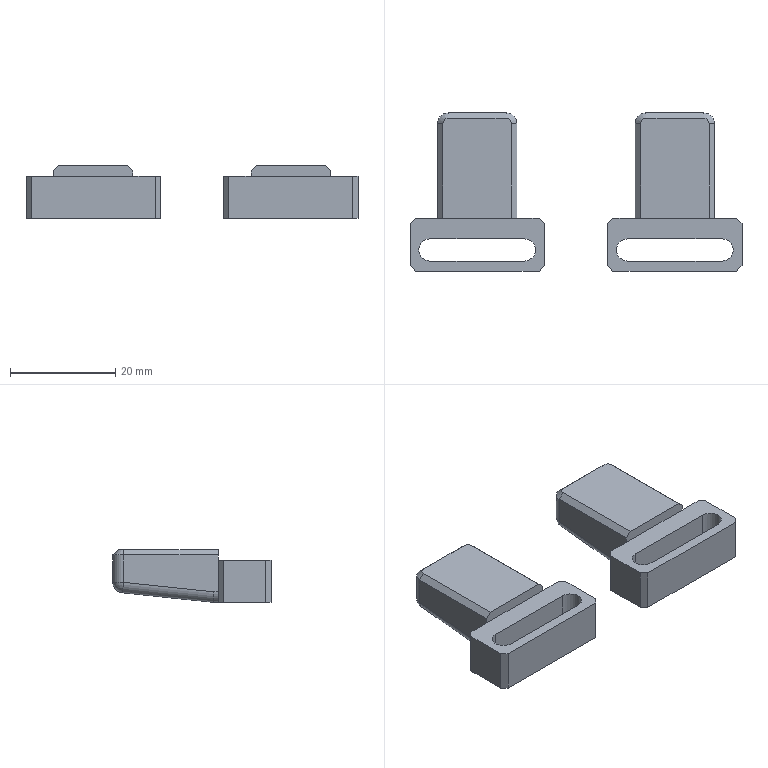NC program | NX | posted with a generic post | part box 63 x 30 x 10 mm
Lines 14606 to 15440 of 24780:
(FIXED_CONTOUR_COPY , TOOL : R2)
N29192 T18 M6
N29194 G54
N29196 G17 G0 G90 X21.594 Y2.999 B0. C0. S9500 M3
N29198 G43 Z30. H18
N29200 Z2.8
N29202 G94 G1 Z-1.939 F1000.
N29204 X21.607 Y2.986 Z-1.906 F2500.
N29206 X21.67 Y2.923 Z-1.669
N29208 X21.669 Y2.857 Z-1.674
N29210 X21.607 Y2.919 Z-1.906
N29212 X21.525 Y3. Z-2.113
N29214 X21.495 Z-2.188
N29216 X21.462 Z-2.252
N29218 Z-2.267
N29220 X21.547 Y2.915 Z-2.061
N29222 X21.607 Y2.855 Z-1.907
N29224 X21.668 Y2.794 Z-1.678
N29226 X21.667 Y2.75 Z-1.68
N29228 X21.607 Y2.811 Z-1.907
N29230 X21.553 Y2.864 Z-2.046
N29232 X21.443 Y2.974 Z-2.311
N29234 X21.418 Y3. Z-2.357
N29236 Z-2.339
N29238 X21.329 Z-2.512
N29240 Y2.999 Z-2.515
N29242 X21.443 Y2.884 Z-2.311
N29244 X21.49 Y2.837 Z-2.199
N29246 X21.565 Y2.762 Z-2.016
N29248 X21.604 Y2.724 Z-1.915
N29250 X21.666 Y2.662 Z-1.686
N29252 X21.665 Y2.596 Z-1.69
N29254 X21.622 Y2.639 Z-1.85
N29256 X21.597 Y2.664 Z-1.932
N29258 X21.566 Y2.695 Z-2.013
N29260 X21.466 Y2.795 Z-2.259
N29262 X21.443 Y2.818 Z-2.311
N29264 X21.284 Y2.977 Z-2.594
N29266 X21.261 Y3. Z-2.627
N29268 Z-2.618
N29270 X21.204 Z-2.701
N29272 Z-2.709
N29274 X21.281 Y2.923 Z-2.599
N29276 X21.443 Y2.761 Z-2.311
N29278 X21.466 Y2.738 Z-2.259
N29280 X21.566 Y2.638 Z-2.014
N29282 X21.592 Y2.613 Z-1.947
N29284 X21.631 Y2.573 Z-1.817
N29286 X21.664 Y2.54 Z-1.694
N29288 X21.663 Y2.438 Z-1.7
N29290 X21.648 Y2.453 Z-1.756
N29292 X21.582 Y2.52 Z-1.973
N29294 X21.466 Y2.635 Z-2.26
N29296 X21.449 Y2.652 Z-2.299
N29298 X21.276 Y2.825 Z-2.609
N29300 X21.194 Y2.907 Z-2.724
N29302 X21.101 Y3. Z-2.85
N29304 Z-2.846
N29306 X21.038 Z-2.92
N29308 Z-2.927
N29310 X21.078 Y2.96 Z-2.881
N29312 X21.194 Y2.844 Z-2.724
N29314 X21.273 Y2.765 Z-2.614
N29316 X21.396 Y2.642 Z-2.393
N29318 X21.453 Y2.585 Z-2.29
N29320 X21.575 Y2.463 Z-1.989
N29322 X21.662 Y2.376 Z-1.704
N29324 X21.66 Y2.273 Z-1.71
N29326 X21.564 Y2.37 Z-2.019
N29328 X21.459 Y2.474 Z-2.276
N29330 X21.369 Y2.564 Z-2.443
N29332 X21.272 Y2.661 Z-2.615
N29334 X21.191 Y2.742 Z-2.728
N29336 X21.078 Y2.855 Z-2.881
N29338 X20.988 Y2.945 Z-2.986
N29340 X20.935 Y2.998 Z-3.042
N29342 X20.898 Z-3.08
N29344 X20.839 Y3. Z-3.136
N29346 Z-3.142
N29348 X20.988 Y2.851 Z-2.986
N29350 X21.078 Y2.761 Z-2.881
N29352 X21.272 Y2.567 Z-2.615
N29354 X21.369 Y2.47 Z-2.443
N29356 X21.465 Y2.374 Z-2.264
N29358 X21.563 Y2.276 Z-2.021
N29360 X21.659 Y2.18 Z-1.716
N29362 X21.657 Y2.078 Z-1.723
N29364 X21.562 Y2.173 Z-2.023
N29366 X21.466 Y2.269 Z-2.262
N29368 X21.369 Y2.366 Z-2.443
N29370 X21.272 Y2.463 Z-2.615
N29372 X21.078 Y2.657 Z-2.881
N29374 X20.987 Y2.748 Z-2.987
N29376 X20.788 Y2.947 Z-3.196
N29378 X20.735 Y3. Z-3.239
N29380 X20.633 Y2.998 Z-3.323
N29382 X20.788 Y2.843 Z-3.196
N29384 X20.966 Y2.666 Z-3.01
N29386 X21.078 Y2.553 Z-2.881
N29388 X21.272 Y2.359 Z-2.615
N29390 X21.399 Y2.232 Z-2.388
N29392 X21.466 Y2.165 Z-2.262
N29394 X21.562 Y2.07 Z-2.025
N29396 X21.656 Y1.975 Z-1.729
N29398 X21.654 Y1.872 Z-1.736
N29400 X21.561 Y1.966 Z-2.026
N29402 X21.466 Y2.06 Z-2.263
N29404 X21.369 Y2.157 Z-2.443
N29406 X21.272 Y2.254 Z-2.615
N29408 X21.078 Y2.449 Z-2.881
N29410 X20.944 Y2.583 Z-3.032
N29412 X20.786 Y2.741 Z-3.198
N29414 X20.548 Y2.978 Z-3.392
N29416 X20.528 Y2.998 Z-3.407
N29418 X20.507 Y3. Z-3.422
N29420 X20.434 Z-3.468
N29422 Z-3.474
N29424 X20.548 Y2.885 Z-3.392
N29426 X20.767 Y2.666 Z-3.213
N29428 X20.822 Y2.611 Z-3.16
N29430 X20.925 Y2.509 Z-3.053
N29432 X21.078 Y2.355 Z-2.88
N29434 X21.272 Y2.161 Z-2.616
N29436 X21.369 Y2.064 Z-2.443
N29438 X21.466 Y1.967 Z-2.264
N29440 X21.56 Y1.873 Z-2.028
N29442 X21.653 Y1.781 Z-1.742
N29444 X21.652 Y1.697 Z-1.747
N29446 X21.56 Y1.789 Z-2.03
N29448 X21.466 Y1.883 Z-2.264
N29450 X21.369 Y1.98 Z-2.443
N29452 X21.272 Y2.077 Z-2.616
N29454 X21.078 Y2.271 Z-2.881
N29456 X20.907 Y2.442 Z-3.071
N29458 X20.849 Y2.5 Z-3.132
N29460 X20.75 Y2.598 Z-3.227
N29462 X20.548 Y2.8 Z-3.392
N29464 X20.471 Y2.878 Z-3.45
N29466 X20.349 Y3. Z-3.527
N29468 Z-3.52
N29470 X20.264 Z-3.573
N29472 Z-3.58
N29474 X20.492 Y2.772 Z-3.437
N29476 X20.734 Y2.53 Z-3.241
N29478 X20.889 Y2.375 Z-3.09
N29480 X21.078 Y2.186 Z-2.881
N29482 X21.272 Y1.992 Z-2.616
N29484 X21.389 Y1.875 Z-2.406
N29486 X21.466 Y1.798 Z-2.264
N29488 X21.559 Y1.705 Z-2.031
N29490 X21.65 Y1.614 Z-1.752
N29492 X21.649 Y1.511 Z-1.759
N29494 X21.558 Y1.601 Z-2.033
N29496 X21.466 Y1.694 Z-2.265
N29498 X21.369 Y1.791 Z-2.443
N29500 X21.272 Y1.888 Z-2.616
N29502 X21.078 Y2.082 Z-2.881
N29504 X20.884 Y2.276 Z-3.095
N29506 X20.713 Y2.447 Z-3.258
N29508 X20.496 Y2.664 Z-3.435
N29510 X20.189 Y2.971 Z-3.627
N29512 X20.16 Y3. Z-3.641
N29514 Z-3.638
N29516 X20.131 Y2.998 Z-3.654
N29518 X20.056 Y3. Z-3.688
N29520 Z-3.69
N29522 X20.189 Y2.867 Z-3.627
N29524 X20.496 Y2.56 Z-3.435
N29526 X20.701 Y2.354 Z-3.266
N29528 X20.884 Y2.171 Z-3.095
N29530 X21.078 Y1.977 Z-2.881
N29532 X21.272 Y1.783 Z-2.616
N29534 X21.369 Y1.686 Z-2.443
N29536 X21.466 Y1.589 Z-2.265
N29538 X21.558 Y1.498 Z-2.035
N29540 X21.647 Y1.408 Z-1.765
N29542 X21.646 Y1.319 Z-1.771
N29544 X21.557 Y1.408 Z-2.036
N29546 X21.466 Y1.499 Z-2.265
N29548 X21.369 Y1.596 Z-2.443
N29550 X21.272 Y1.693 Z-2.616
N29552 X21.078 Y1.887 Z-2.881
N29554 X20.884 Y2.081 Z-3.095
N29556 X20.69 Y2.275 Z-3.276
N29558 X20.496 Y2.469 Z-3.435
N29560 X20.189 Y2.776 Z-3.627
N29562 X19.965 Y3. Z-3.732
N29564 Z-3.726
N29566 X19.874 Z-3.765
N29568 Z-3.774
N29570 X20.178 Y2.696 Z-3.633
N29572 X20.215 Y2.659 Z-3.611
N29574 X20.496 Y2.378 Z-3.435
N29576 X20.69 Y2.184 Z-3.276
N29578 X20.884 Y1.99 Z-3.095
N29580 X21.078 Y1.796 Z-2.881
N29582 X21.272 Y1.602 Z-2.616
N29584 X21.369 Y1.505 Z-2.443
N29586 X21.466 Y1.408 Z-2.266
N29588 X21.556 Y1.318 Z-2.038
N29590 X21.645 Y1.229 Z-1.776
N29592 X21.643 Y1.127 Z-1.783
N29594 X21.555 Y1.215 Z-2.04
N29596 X21.466 Y1.304 Z-2.266
N29598 X21.338 Y1.432 Z-2.499
N29600 X21.272 Y1.498 Z-2.616
N29602 X21.078 Y1.692 Z-2.881
N29604 X20.884 Y1.886 Z-3.095
N29606 X20.69 Y2.08 Z-3.276
N29608 X20.496 Y2.274 Z-3.435
N29610 X20.257 Y2.513 Z-3.585
N29612 X20.16 Y2.61 Z-3.641
N29614 X19.914 Y2.856 Z-3.757
N29616 X19.824 Y2.946 Z-3.796
N29618 X19.77 Y3. Z-3.813
N29620 Z-3.809
N29622 X19.737 Y2.998 Z-3.824
N29624 X19.711 Y3. Z-3.832
N29626 X19.667 Z-3.843
N29628 Z-3.846
N29630 X19.824 Y2.842 Z-3.796
N29632 X19.915 Y2.751 Z-3.756
N29634 X20.142 Y2.524 Z-3.65
N29636 X20.298 Y2.368 Z-3.559
N29638 X20.496 Y2.17 Z-3.435
N29640 X20.69 Y1.976 Z-3.276
N29642 X20.884 Y1.782 Z-3.095
N29644 X21.078 Y1.588 Z-2.881
N29646 X21.272 Y1.394 Z-2.616
N29648 X21.466 Y1.2 Z-2.266
N29650 X21.555 Y1.112 Z-2.042
N29652 X21.642 Y1.024 Z-1.789
N29654 X21.64 Y0.931 Z-1.795
N29656 X21.554 Y1.017 Z-2.044
N29658 X21.466 Y1.105 Z-2.266
N29660 X21.272 Y1.299 Z-2.617
N29662 X21.078 Y1.493 Z-2.881
N29664 X20.884 Y1.687 Z-3.095
N29666 X20.69 Y1.881 Z-3.276
N29668 X20.496 Y2.075 Z-3.435
N29670 X20.302 Y2.269 Z-3.556
N29672 X20.126 Y2.445 Z-3.657
N29674 X19.914 Y2.657 Z-3.757
N29676 X19.883 Y2.688 Z-3.768
N29678 X19.823 Y2.748 Z-3.796
N29680 X19.571 Y3. Z-3.877
N29682 Z-3.869
N29684 X19.475 Z-3.895
N29686 Z-3.904
N29688 X19.526 Y2.949 Z-3.892
N29690 X19.803 Y2.672 Z-3.803
N29692 X19.851 Y2.623 Z-3.78
N29694 X19.914 Y2.561 Z-3.757
N29696 X20.12 Y2.354 Z-3.659
N29698 X20.302 Y2.173 Z-3.556
N29700 X20.496 Y1.979 Z-3.435
N29702 X20.69 Y1.785 Z-3.276
N29704 X20.884 Y1.591 Z-3.095
N29706 X21.078 Y1.397 Z-2.881
N29708 X21.272 Y1.203 Z-2.617
N29710 X21.466 Y1.008 Z-2.266
N29712 X21.553 Y0.922 Z-2.045
N29714 X21.639 Y0.836 Z-1.801
N29716 X21.638 Y0.733 Z-1.808
N29718 X21.552 Y0.819 Z-2.047
N29720 X21.466 Y0.905 Z-2.266
N29722 X21.272 Y1.099 Z-2.617
N29724 X21.078 Y1.293 Z-2.881
N29726 X20.884 Y1.487 Z-3.095
N29728 X20.69 Y1.681 Z-3.276
N29730 X20.496 Y1.875 Z-3.435
N29732 X20.302 Y2.069 Z-3.556
N29734 X20.108 Y2.263 Z-3.666
N29736 X19.914 Y2.457 Z-3.757
N29738 X19.817 Y2.554 Z-3.793
N29740 X19.781 Y2.59 Z-3.809
N29742 X19.526 Y2.845 Z-3.892
N29744 X19.436 Y2.935 Z-3.914
N29746 X19.371 Y3. Z-3.926
N29748 Z-3.923
N29750 X19.342 Y2.998 Z-3.931
N29752 X19.307 Y3. Z-3.938
N29754 X19.268 Z-3.943
N29756 Z-3.945
N29758 X19.436 Y2.832 Z-3.914
N29760 X19.526 Y2.742 Z-3.892
N29762 X19.76 Y2.508 Z-3.816
N29764 X19.783 Y2.484 Z-3.806
N29766 X19.914 Y2.353 Z-3.756
N29768 X20.108 Y2.16 Z-3.666
N29770 X20.302 Y1.966 Z-3.556
N29772 X20.496 Y1.772 Z-3.435
N29774 X20.69 Y1.578 Z-3.276
N29776 X20.884 Y1.383 Z-3.095
N29778 X21.078 Y1.189 Z-2.881
N29780 X21.272 Y0.995 Z-2.617
N29782 X21.466 Y0.801 Z-2.266
N29784 X21.552 Y0.716 Z-2.049
N29786 X21.636 Y0.631 Z-1.814
N29788 X21.635 Y0.535 Z-1.82
N29790 X21.551 Y0.618 Z-2.051
N29792 X21.466 Y0.703 Z-2.266
N29794 X21.272 Y0.897 Z-2.618
N29796 X21.078 Y1.091 Z-2.881
N29798 X20.884 Y1.285 Z-3.095
N29800 X20.69 Y1.479 Z-3.276
N29802 X20.496 Y1.673 Z-3.435
N29804 X20.302 Y1.867 Z-3.556
N29806 X20.108 Y2.061 Z-3.666
N29808 X19.914 Y2.256 Z-3.757
N29810 X19.739 Y2.43 Z-3.823
N29812 X19.526 Y2.644 Z-3.892
N29814 X19.432 Y2.737 Z-3.914
N29816 X19.17 Y3. Z-3.964
N29818 Z-3.958
N29820 X19.071 Z-3.973
N29822 Z-3.978
N29824 X19.138 Y2.933 Z-3.97
N29826 X19.411 Y2.659 Z-3.918
N29828 X19.526 Y2.545 Z-3.892
N29830 X19.72 Y2.351 Z-3.829
N29832 X19.914 Y2.157 Z-3.757
N29834 X20.108 Y1.963 Z-3.666
N29836 X20.302 Y1.768 Z-3.556
N29838 X20.496 Y1.574 Z-3.435
N29840 X20.69 Y1.38 Z-3.276
N29842 X20.884 Y1.186 Z-3.095
N29844 X21.078 Y0.992 Z-2.881
N29846 X21.272 Y0.798 Z-2.618
N29848 X21.466 Y0.604 Z-2.266
N29850 X21.55 Y0.52 Z-2.053
N29852 X21.633 Y0.437 Z-1.827
N29854 X21.632 Y0.335 Z-1.833
N29856 X21.549 Y0.417 Z-2.055
N29858 X21.466 Y0.501 Z-2.266
N29860 X21.272 Y0.695 Z-2.618
N29862 X21.078 Y0.889 Z-2.881
N29864 X20.884 Y1.083 Z-3.095
N29866 X20.69 Y1.277 Z-3.276
N29868 X20.496 Y1.471 Z-3.435
N29870 X20.302 Y1.665 Z-3.556
N29872 X20.108 Y1.859 Z-3.666
N29874 X19.914 Y2.053 Z-3.757
N29876 X19.72 Y2.247 Z-3.829
N29878 X19.526 Y2.441 Z-3.892
N29880 X19.39 Y2.577 Z-3.922
N29882 X19.138 Y2.829 Z-3.97
N29884 X18.967 Y3. Z-3.99
N29886 X18.918 Z-3.992
N29888 X18.863
N29890 Z-3.995
N29892 X18.985 Y2.877 Z-3.989
N29894 X19.138 Y2.725 Z-3.97
N29896 X19.368 Y2.494 Z-3.926
N29898 X19.526 Y2.337 Z-3.892
N29900 X19.72 Y2.143 Z-3.829
N29902 X19.914 Y1.949 Z-3.757
N29904 X20.108 Y1.755 Z-3.666
N29906 X20.303 Y1.56 Z-3.556
N29908 X20.496 Y1.367 Z-3.435
N29910 X20.69 Y1.173 Z-3.276
N29912 X20.884 Y0.979 Z-3.095
N29914 X21.078 Y0.785 Z-2.881
N29916 X21.272 Y0.591 Z-2.618
N29918 X21.466 Y0.397 Z-2.266
N29920 X21.549 Y0.314 Z-2.058
N29922 X21.63 Y0.233 Z-1.839
N29924 X21.628 Y0.135 Z-1.845
N29926 X21.548 Y0.215 Z-2.061
N29928 X21.466 Y0.297 Z-2.266
N29930 X21.272 Y0.491 Z-2.618
N29932 X21.078 Y0.685 Z-2.881
N29934 X20.884 Y0.879 Z-3.095
N29936 X20.69 Y1.073 Z-3.276
N29938 X20.496 Y1.267 Z-3.435
N29940 X20.302 Y1.461 Z-3.556
N29942 X20.108 Y1.655 Z-3.666
N29944 X19.914 Y1.849 Z-3.757
N29946 X19.72 Y2.043 Z-3.829
N29948 X19.526 Y2.237 Z-3.892
N29950 X19.348 Y2.415 Z-3.93
N29952 X19.138 Y2.625 Z-3.97
N29954 X18.953 Y2.81 Z-3.992
N29956 X18.763 Y3. Z-3.999
N29958 Z-3.992
N29960 X18.663
N29962 Z-3.996
N29964 X18.749 Y2.913 Z-3.999
N29966 X18.943 Y2.719 Z-3.993
N29968 X19.138 Y2.525 Z-3.97
N29970 X19.332 Y2.331 Z-3.933
N29972 X19.526 Y2.137 Z-3.892
N29974 X19.72 Y1.943 Z-3.829
N29976 X19.914 Y1.749 Z-3.757
N29978 X20.108 Y1.555 Z-3.666
N29980 X20.302 Y1.361 Z-3.556
N29982 X20.496 Y1.167 Z-3.435
N29984 X20.69 Y0.973 Z-3.276
N29986 X20.884 Y0.779 Z-3.095
N29988 X21.078 Y0.585 Z-2.881
N29990 X21.272 Y0.391 Z-2.619
N29992 X21.466 Y0.197 Z-2.266
N29994 X21.547 Y0.116 Z-2.064
N29996 X21.626 Y0.037 Z-1.852
N29998 X21.624 Y-0.066 Z-1.858
N30000 X21.535 Y0.023 Z-2.094
N30002 X21.466 Y0.091 Z-2.266
N30004 X21.272 Y0.286 Z-2.619
N30006 X21.078 Y0.48 Z-2.881
N30008 X20.884 Y0.674 Z-3.095
N30010 X20.69 Y0.868 Z-3.276
N30012 X20.496 Y1.062 Z-3.435
N30014 X20.302 Y1.256 Z-3.556
N30016 X20.108 Y1.45 Z-3.666
N30018 X19.914 Y1.644 Z-3.757
N30020 X19.72 Y1.838 Z-3.829
N30022 X19.526 Y2.032 Z-3.892
N30024 X19.332 Y2.226 Z-3.933
N30026 X19.138 Y2.42 Z-3.97
N30028 X18.943 Y2.614 Z-3.993
N30030 X18.749 Y2.808 Z-3.999
N30032 X18.559 Y2.998 Z-3.991
N30034 X18.532 Y3. Z-3.989
N30036 X18.452 Z-3.977
N30038 Z-3.981
N30040 X18.526 Y2.926 Z-3.99
N30042 X18.656 Y2.796 Z-3.996
N30044 X18.749 Y2.703 Z-3.999
N30046 X18.958 Y2.494 Z-3.991
N30048 X19.138 Y2.315 Z-3.97
N30050 X19.332 Y2.121 Z-3.933
N30052 X19.526 Y1.926 Z-3.892
N30054 X19.72 Y1.732 Z-3.829
N30056 X19.914 Y1.538 Z-3.757
N30058 X20.108 Y1.344 Z-3.666
N30060 X20.302 Y1.15 Z-3.556
N30062 X20.496 Y0.956 Z-3.435
N30064 X20.69 Y0.762 Z-3.276
N30066 X20.884 Y0.568 Z-3.095
N30068 X21.078 Y0.374 Z-2.881
N30070 X21.272 Y0.18 Z-2.619
N30072 X21.466 Y-0.014 Z-2.266
N30074 X21.559 Y-0.107 Z-2.032
N30076 X21.622 Y-0.169 Z-1.865
N30078 X21.62 Y-0.273 Z-1.871
N30080 X21.544 Y-0.197 Z-2.074
N30082 X21.466 Y-0.12 Z-2.266
N30084 X21.272 Y0.074 Z-2.619
N30086 X21.078 Y0.268 Z-2.881
N30088 X20.884 Y0.463 Z-3.095
N30090 X20.69 Y0.657 Z-3.276
N30092 X20.496 Y0.851 Z-3.435
N30094 X20.302 Y1.045 Z-3.556
N30096 X20.108 Y1.239 Z-3.666
N30098 X19.914 Y1.433 Z-3.757
N30100 X19.72 Y1.627 Z-3.829
N30102 X19.526 Y1.821 Z-3.892
N30104 X19.332 Y2.015 Z-3.933
N30106 X19.138 Y2.209 Z-3.97
N30108 X18.943 Y2.403 Z-3.993
N30110 X18.749 Y2.597 Z-3.999
N30112 X18.547 Y2.799 Z-3.992
N30114 X18.347 Y3. Z-3.967
N30116 Z-3.961
N30118 X18.241 Z-3.944
N30120 Z-3.947
N30122 X18.361 Y2.88 Z-3.97
N30124 X18.555 Y2.686 Z-3.992
N30126 X18.749 Y2.492 Z-3.999
N30128 X18.943 Y2.298 Z-3.993
N30130 X19.138 Y2.103 Z-3.97
N30132 X19.332 Y1.909 Z-3.933
N30134 X19.526 Y1.715 Z-3.892
N30136 X19.72 Y1.521 Z-3.829
N30138 X19.914 Y1.327 Z-3.757
N30140 X20.108 Y1.133 Z-3.666
N30142 X20.302 Y0.939 Z-3.556
N30144 X20.496 Y0.745 Z-3.435
N30146 X20.69 Y0.551 Z-3.276
N30148 X20.884 Y0.357 Z-3.095
N30150 X21.078 Y0.163 Z-2.881
N30152 X21.272 Y-0.031 Z-2.619
N30154 X21.466 Y-0.225 Z-2.266
N30156 X21.543 Y-0.302 Z-2.078
N30158 X21.617 Y-0.376 Z-1.878
N30160 X21.615 Y-0.48 Z-1.884
N30162 X21.541 Y-0.406 Z-2.081
N30164 X21.466 Y-0.331 Z-2.266
N30166 X21.272 Y-0.137 Z-2.619
N30168 X21.078 Y0.057 Z-2.881
N30170 X20.884 Y0.251 Z-3.095
N30172 X20.69 Y0.445 Z-3.276
N30174 X20.496 Y0.639 Z-3.435
N30176 X20.302 Y0.833 Z-3.556
N30178 X20.108 Y1.027 Z-3.666
N30180 X19.914 Y1.221 Z-3.757
N30182 X19.72 Y1.416 Z-3.829
N30184 X19.526 Y1.61 Z-3.892
N30186 X19.332 Y1.804 Z-3.933
N30188 X19.138 Y1.998 Z-3.97
N30190 X18.943 Y2.192 Z-3.993
N30192 X18.749 Y2.386 Z-3.999
N30194 X18.555 Y2.58 Z-3.992
N30196 X18.361 Y2.774 Z-3.97
N30198 X18.136 Y3. Z-3.927
N30200 Z-3.925
N30202 X18.036 Z-3.898
N30204 Z-3.907
N30206 X18.063 Y2.972 Z-3.913
N30208 X18.361 Y2.674 Z-3.97
N30210 X18.555 Y2.48 Z-3.992
N30212 X18.749 Y2.286 Z-3.999
N30214 X18.943 Y2.092 Z-3.993
N30216 X19.138 Y1.898 Z-3.97
N30218 X19.332 Y1.704 Z-3.933
N30220 X19.526 Y1.51 Z-3.892
N30222 X19.72 Y1.316 Z-3.829
N30224 X19.914 Y1.121 Z-3.757
N30226 X20.108 Y0.927 Z-3.666
N30228 X20.302 Y0.733 Z-3.556
N30230 X20.496 Y0.539 Z-3.435
N30232 X20.69 Y0.345 Z-3.276
N30234 X20.884 Y0.151 Z-3.095
N30236 X21.078 Y-0.043 Z-2.881
N30238 X21.272 Y-0.237 Z-2.619
N30240 X21.466 Y-0.431 Z-2.266
N30242 X21.54 Y-0.505 Z-2.084
N30244 X21.613 Y-0.578 Z-1.891
N30246 X21.612 Y-0.676 Z-1.897
N30248 X21.54 Y-0.604 Z-2.088
N30250 X21.466 Y-0.531 Z-2.267
N30252 X21.272 Y-0.337 Z-2.619
N30254 X21.078 Y-0.143 Z-2.881
N30256 X20.884 Y0.051 Z-3.095
N30258 X20.69 Y0.245 Z-3.276
N30260 X20.496 Y0.439 Z-3.435
N30262 X20.302 Y0.633 Z-3.556
N30264 X20.108 Y0.827 Z-3.666
N30266 X19.914 Y1.021 Z-3.757
N30268 X19.72 Y1.216 Z-3.829
N30270 X19.526 Y1.41 Z-3.892
N30272 X19.332 Y1.604 Z-3.933
N30274 X19.138 Y1.798 Z-3.97
N30276 X18.943 Y1.992 Z-3.993
N30278 X18.749 Y2.186 Z-3.999
N30280 X18.555 Y2.38 Z-3.992
N30282 X18.361 Y2.574 Z-3.97
N30284 X18.063 Y2.872 Z-3.913
N30286 X17.973 Y2.962 Z-3.891
N30288 X17.936 Y3. Z-3.879
N30290 Z-3.871
N30292 X17.836 Z-3.844
N30294 Z-3.847
N30296 X17.973 Y2.862 Z-3.891
N30298 X18.084 Y2.751 Z-3.917
N30300 X18.361 Y2.474 Z-3.97
N30302 X18.555 Y2.28 Z-3.992
N30304 X18.749 Y2.086 Z-3.999
N30306 X18.943 Y1.892 Z-3.993
N30308 X19.138 Y1.698 Z-3.97
N30310 X19.332 Y1.504 Z-3.933
N30312 X19.526 Y1.31 Z-3.892
N30314 X19.72 Y1.116 Z-3.829
N30316 X19.914 Y0.921 Z-3.757
N30318 X20.108 Y0.727 Z-3.666
N30320 X20.302 Y0.533 Z-3.556
N30322 X20.496 Y0.339 Z-3.435
N30324 X20.69 Y0.145 Z-3.276
N30326 X20.884 Y-0.049 Z-3.095
N30328 X21.078 Y-0.243 Z-2.881
N30330 X21.272 Y-0.437 Z-2.619
N30332 X21.466 Y-0.631 Z-2.267
N30334 X21.539 Y-0.703 Z-2.091
N30336 X21.609 Y-0.774 Z-1.903
N30338 X21.608 Y-0.878 Z-1.909
N30340 X21.537 Y-0.808 Z-2.094
N30342 X21.466 Y-0.737 Z-2.267
N30344 X21.272 Y-0.543 Z-2.619
N30346 X21.078 Y-0.349 Z-2.881
N30348 X20.884 Y-0.155 Z-3.095
N30350 X20.69 Y0.039 Z-3.276
N30352 X20.496 Y0.233 Z-3.435
N30354 X20.302 Y0.428 Z-3.556
N30356 X20.108 Y0.622 Z-3.666
N30358 X19.914 Y0.816 Z-3.757
N30360 X19.72 Y1.01 Z-3.829
N30362 X19.526 Y1.204 Z-3.892
N30364 X19.332 Y1.398 Z-3.933
N30366 X19.138 Y1.592 Z-3.97
N30368 X18.943 Y1.786 Z-3.993
N30370 X18.749 Y1.98 Z-3.999
N30372 X18.555 Y2.174 Z-3.992
N30374 X18.361 Y2.368 Z-3.97
N30376 X18.047 Y2.682 Z-3.91
N30378 X17.974 Y2.755 Z-3.892
N30380 X17.73 Y3. Z-3.813
N30382 Z-3.81
N30384 X17.63 Z-3.767
N30386 Z-3.776
N30388 X17.675 Y2.954 Z-3.795
N30390 X17.973 Y2.656 Z-3.891
N30392 X18.029 Y2.6 Z-3.905
N30394 X18.361 Y2.268 Z-3.97
N30396 X18.555 Y2.074 Z-3.992
N30398 X18.749 Y1.88 Z-3.999
N30400 X18.943 Y1.686 Z-3.993
N30402 X19.138 Y1.492 Z-3.97
N30404 X19.332 Y1.298 Z-3.933
N30406 X19.526 Y1.104 Z-3.892
N30408 X19.72 Y0.91 Z-3.829
N30410 X19.914 Y0.716 Z-3.757
N30412 X20.108 Y0.522 Z-3.666
N30414 X20.302 Y0.328 Z-3.556
N30416 X20.496 Y0.133 Z-3.435
N30418 X20.69 Y-0.061 Z-3.276
N30420 X20.884 Y-0.255 Z-3.095
N30422 X21.078 Y-0.449 Z-2.881
N30424 X21.272 Y-0.643 Z-2.619
N30426 X21.466 Y-0.837 Z-2.267
N30428 X21.536 Y-0.907 Z-2.098
N30430 X21.606 Y-0.976 Z-1.916
N30432 X21.604 Y-1.074 Z-1.922
N30434 X21.535 Y-1.006 Z-2.101
N30436 X21.466 Y-0.937 Z-2.267
N30438 X21.272 Y-0.743 Z-2.619
N30440 X21.078 Y-0.549 Z-2.881
N30442 X20.884 Y-0.355 Z-3.095
N30444 X20.69 Y-0.161 Z-3.276
N30446 X20.496 Y0.034 Z-3.435
N30448 X20.302 Y0.228 Z-3.556
N30450 X20.108 Y0.422 Z-3.666
N30452 X19.914 Y0.616 Z-3.757
N30454 X19.72 Y0.81 Z-3.829
N30456 X19.526 Y1.004 Z-3.892
N30458 X19.332 Y1.198 Z-3.933
N30460 X19.138 Y1.392 Z-3.97
N30462 X18.943 Y1.586 Z-3.993
N30464 X18.749 Y1.78 Z-3.999
N30466 X18.555 Y1.974 Z-3.992
N30468 X18.361 Y2.168 Z-3.97
N30470 X18.17 Y2.36 Z-3.934
N30472 X17.973 Y2.556 Z-3.891
N30474 X17.675 Y2.854 Z-3.795
N30476 X17.53 Y3. Z-3.73
N30478 Z-3.724
N30480 X17.43 Z-3.682
N30482 Z-3.684
N30484 X17.585 Y2.844 Z-3.756
N30486 X17.676 Y2.754 Z-3.796
N30488 X17.973 Y2.456 Z-3.891
N30490 X18.167 Y2.262 Z-3.933
N30492 X18.361 Y2.068 Z-3.97
N30494 X18.555 Y1.874 Z-3.992
N30496 X18.749 Y1.68 Z-3.999
N30498 X18.943 Y1.486 Z-3.993
N30500 X19.138 Y1.292 Z-3.97
N30502 X19.332 Y1.098 Z-3.933
N30504 X19.526 Y0.904 Z-3.892
N30506 X19.72 Y0.71 Z-3.829
N30508 X19.914 Y0.516 Z-3.757
N30510 X20.108 Y0.322 Z-3.666
N30512 X20.302 Y0.128 Z-3.556
N30514 X20.496 Y-0.066 Z-3.435
N30516 X20.69 Y-0.26 Z-3.276
N30518 X20.884 Y-0.455 Z-3.095
N30520 X21.078 Y-0.649 Z-2.881
N30522 X21.272 Y-0.843 Z-2.619
N30524 X21.466 Y-1.037 Z-2.267
N30526 X21.534 Y-1.105 Z-2.104
N30528 X21.602 Y-1.172 Z-1.928
N30530 X21.599 Y-1.276 Z-1.934
N30532 X21.533 Y-1.21 Z-2.107
N30534 X21.466 Y-1.142 Z-2.267
N30536 X21.272 Y-0.948 Z-2.619
N30538 X21.078 Y-0.754 Z-2.881
N30540 X20.884 Y-0.56 Z-3.095
N30542 X20.69 Y-0.366 Z-3.276
N30544 X20.496 Y-0.172 Z-3.435
N30546 X20.302 Y0.022 Z-3.556
N30548 X20.108 Y0.216 Z-3.666
N30550 X19.914 Y0.41 Z-3.757
N30552 X19.72 Y0.604 Z-3.829
N30554 X19.526 Y0.798 Z-3.892
N30556 X19.332 Y0.992 Z-3.933
N30558 X19.138 Y1.186 Z-3.97
N30560 X18.943 Y1.38 Z-3.993
N30562 X18.749 Y1.574 Z-3.999
N30564 X18.555 Y1.768 Z-3.992
N30566 X18.361 Y1.963 Z-3.97
N30568 X18.167 Y2.157 Z-3.933
N30570 X17.973 Y2.351 Z-3.891
N30572 X17.712 Y2.612 Z-3.807
N30574 X17.656 Y2.668 Z-3.787
N30576 X17.585 Y2.739 Z-3.756
N30578 X17.324 Y3. Z-3.634
N30580 Z-3.628
N30582 X17.218 Z-3.562
N30584 Z-3.569
N30586 X17.311 Y2.907 Z-3.627
N30588 X17.585 Y2.633 Z-3.756
N30590 X17.637 Y2.581 Z-3.779
N30592 X17.749 Y2.469 Z-3.819
N30594 X17.973 Y2.245 Z-3.891
N30596 X18.167 Y2.051 Z-3.933
N30598 X18.361 Y1.857 Z-3.97
N30600 X18.555 Y1.663 Z-3.992
N30602 X18.749 Y1.469 Z-3.999
N30604 X18.943 Y1.275 Z-3.993
N30606 X19.138 Y1.08 Z-3.97
N30608 X19.332 Y0.886 Z-3.933
N30610 X19.526 Y0.692 Z-3.892
N30612 X19.72 Y0.498 Z-3.829
N30614 X19.914 Y0.304 Z-3.757
N30616 X20.108 Y0.11 Z-3.666
N30618 X20.302 Y-0.084 Z-3.556
N30620 X20.496 Y-0.278 Z-3.435
N30622 X20.69 Y-0.472 Z-3.276
N30624 X20.884 Y-0.666 Z-3.095
N30626 X21.078 Y-0.86 Z-2.881
N30628 X21.272 Y-1.054 Z-2.619
N30630 X21.466 Y-1.248 Z-2.267
N30632 X21.55 Y-1.332 Z-2.065
N30634 X21.597 Y-1.379 Z-1.941
N30636 X21.595 Y-1.483 Z-1.947
N30638 X21.504 Y-1.392 Z-2.177
N30640 X21.466 Y-1.354 Z-2.267
N30642 X21.272 Y-1.16 Z-2.619
N30644 X21.078 Y-0.966 Z-2.881
N30646 X20.884 Y-0.772 Z-3.095
N30648 X20.69 Y-0.578 Z-3.276
N30650 X20.496 Y-0.384 Z-3.435
N30652 X20.302 Y-0.19 Z-3.556
N30654 X20.108 Y0.004 Z-3.666
N30656 X19.914 Y0.198 Z-3.757
N30658 X19.72 Y0.393 Z-3.829
N30660 X19.526 Y0.587 Z-3.892
N30662 X19.332 Y0.781 Z-3.933
N30664 X19.138 Y0.975 Z-3.97
N30666 X18.943 Y1.169 Z-3.993
N30668 X18.749 Y1.363 Z-3.999
N30670 X18.555 Y1.557 Z-3.992
N30672 X18.361 Y1.751 Z-3.97
N30674 X18.167 Y1.945 Z-3.933
N30676 X17.973 Y2.139 Z-3.891
N30678 X17.758 Y2.354 Z-3.821
N30680 X17.617 Y2.495 Z-3.77
N30682 X17.311 Y2.801 Z-3.627
N30684 X17.113 Y3. Z-3.503
N30686 Z-3.496
N30688 X17.007 Z-3.431
N30690 X17.052 Y2.954 Z-3.465
N30692 X17.255 Y2.751 Z-3.592
N30694 X17.325 Y2.682 Z-3.634
N30696 X17.598 Y2.409 Z-3.762
N30698 X17.779 Y2.228 Z-3.829
N30700 X17.973 Y2.034 Z-3.891
N30702 X18.167 Y1.84 Z-3.933
N30704 X18.361 Y1.645 Z-3.97
N30706 X18.555 Y1.451 Z-3.992
N30708 X18.749 Y1.257 Z-3.999
N30710 X18.943 Y1.063 Z-3.993
N30712 X19.138 Y0.869 Z-3.97
N30714 X19.332 Y0.675 Z-3.933
N30716 X19.526 Y0.481 Z-3.892
N30718 X19.72 Y0.287 Z-3.829
N30720 X19.914 Y0.093 Z-3.757
N30722 X20.108 Y-0.101 Z-3.666
N30724 X20.302 Y-0.295 Z-3.556
N30726 X20.496 Y-0.489 Z-3.435
N30728 X20.69 Y-0.683 Z-3.276
N30730 X20.884 Y-0.877 Z-3.095
N30732 X21.078 Y-1.071 Z-2.881
N30734 X21.272 Y-1.265 Z-2.619
N30736 X21.466 Y-1.459 Z-2.267
N30738 X21.593 Y-1.586 Z-1.954
N30740 X21.591 Y-1.69 Z-1.96
N30742 X21.466 Y-1.565 Z-2.267
N30744 X21.272 Y-1.371 Z-2.619
N30746 X21.078 Y-1.177 Z-2.881
N30748 X20.884 Y-0.983 Z-3.095
N30750 X20.69 Y-0.789 Z-3.276
N30752 X20.496 Y-0.595 Z-3.435
N30754 X20.302 Y-0.401 Z-3.556
N30756 X20.108 Y-0.207 Z-3.666
N30758 X19.914 Y-0.013 Z-3.757
N30760 X19.72 Y0.181 Z-3.829
N30762 X19.526 Y0.375 Z-3.892
N30764 X19.332 Y0.569 Z-3.933
N30766 X19.138 Y0.763 Z-3.97
N30768 X18.943 Y0.957 Z-3.993
N30770 X18.749 Y1.151 Z-3.999
N30772 X18.555 Y1.345 Z-3.992
N30774 X18.361 Y1.539 Z-3.97
N30776 X18.167 Y1.734 Z-3.933
N30778 X17.973 Y1.928 Z-3.891
N30780 X17.779 Y2.122 Z-3.829
N30782 X17.585 Y2.316 Z-3.756
N30784 X17.352 Y2.549 Z-3.647
N30786 X17.197 Y2.704 Z-3.556
N30788 X17.052 Y2.848 Z-3.465
N30790 X16.964 Y2.937 Z-3.402
N30792 X16.902 Y2.998 Z-3.352
N30794 X16.796 Z-3.265
N30796 X16.992 Y2.803 Z-3.425
N30798 X17.043 Y2.751 Z-3.459
N30800 X17.197 Y2.598 Z-3.556
N30802 X17.378 Y2.416 Z-3.66
N30804 X17.585 Y2.21 Z-3.756
N30806 X17.779 Y2.016 Z-3.829
N30808 X17.973 Y1.822 Z-3.891
N30810 X18.167 Y1.627 Z-3.933
N30812 X18.361 Y1.433 Z-3.97
N30814 X18.555 Y1.239 Z-3.992
N30816 X18.749 Y1.045 Z-3.999
N30818 X18.943 Y0.851 Z-3.993
N30820 X19.138 Y0.657 Z-3.97
N30822 X19.332 Y0.463 Z-3.933
N30824 X19.526 Y0.269 Z-3.892
N30826 X19.72 Y0.075 Z-3.829
N30828 X19.914 Y-0.119 Z-3.757
N30830 X20.108 Y-0.313 Z-3.666
N30832 X20.302 Y-0.507 Z-3.556
N30834 X20.496 Y-0.701 Z-3.435
N30836 X20.69 Y-0.895 Z-3.276
N30838 X20.884 Y-1.089 Z-3.095
N30840 X21.078 Y-1.283 Z-2.881
N30842 X21.272 Y-1.478 Z-2.619
N30844 X21.466 Y-1.672 Z-2.267
N30846 X21.588 Y-1.794 Z-1.967
N30848 X21.586 Y-1.898 Z-1.973
N30850 X21.466 Y-1.778 Z-2.267
N30852 X21.272 Y-1.584 Z-2.619
N30854 X21.078 Y-1.39 Z-2.881